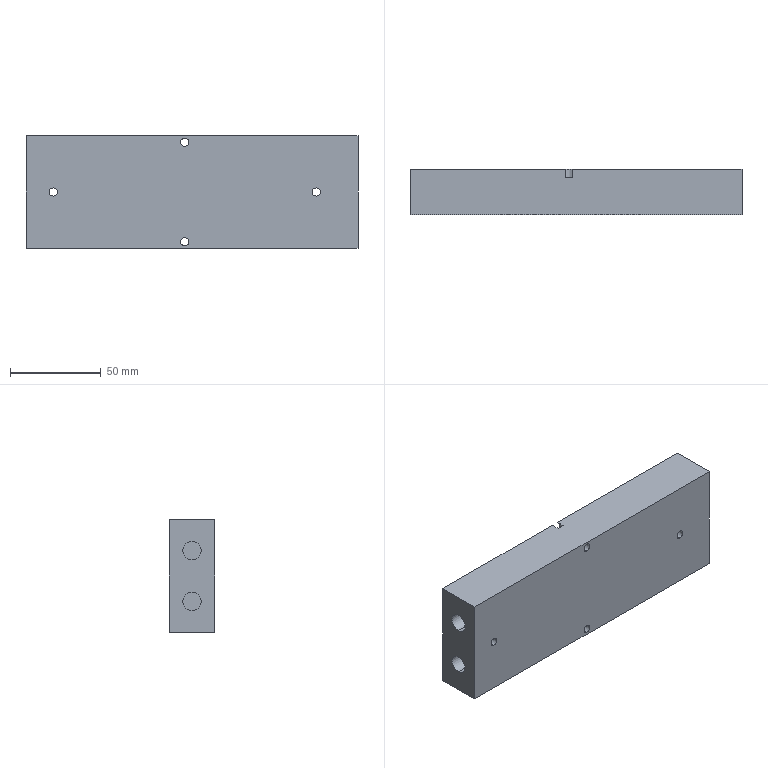Part | STEP file | PN_0014 cylinder TN-20X125 | 1 solid | 31 faces | box 183 x 25 x 62 mm | volume 276727 mm3 | cylinder 19 | plane 12 | commonest cylinder face diameters 4.5 x8 8 x7 10 x4